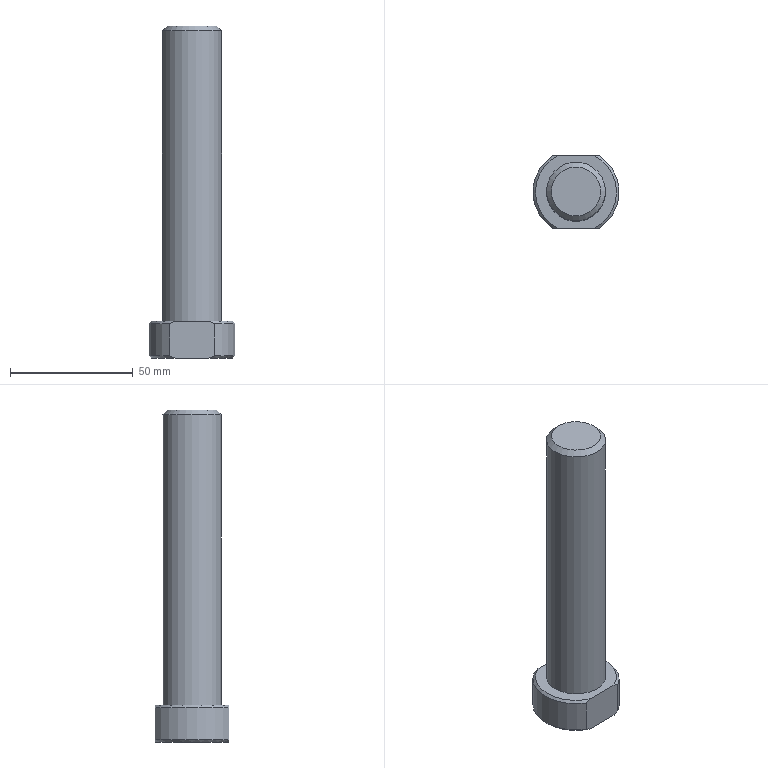Part | NX | features stopper pipe 2 | 1 solid | 13 faces | box 35 x 30 x 135 mm | volume 67591 mm3 | cone 5 | plane 5 | cylinder 3 | commonest cylinder face diameters 35 x2 24 x1
STEP:
#1=CARTESIAN_POINT('',(9.014,-15.,-1.));
#2=VERTEX_POINT('',#1);
#3=CARTESIAN_POINT('',(9.014,15.,-1.));
#4=VERTEX_POINT('',#3);
#5=CARTESIAN_POINT('',(0.,0.,-1.));
#6=DIRECTION('',(0.,0.,-1.));
#7=DIRECTION('',(-1.,0.,0.));
#8=AXIS2_PLACEMENT_3D('',#5,#6,#7);
#9=CIRCLE('',#8,17.5);
#10=EDGE_CURVE('',#2,#4,#9,.F.);
#11=ORIENTED_EDGE('',*,*,#10,.F.);
#12=CARTESIAN_POINT('',(9.014,-15.,-14.));
#13=VERTEX_POINT('',#12);
#14=CARTESIAN_POINT('',(9.014,-15.,120.));
#15=DIRECTION('',(0.,0.,-1.));
#16=VECTOR('',#15,1000.);
#17=LINE('',#14,#16);
#18=EDGE_CURVE('',#13,#2,#17,.F.);
#19=ORIENTED_EDGE('',*,*,#18,.F.);
#20=CARTESIAN_POINT('',(9.014,15.,-14.));
#21=VERTEX_POINT('',#20);
#22=CARTESIAN_POINT('',(0.,0.,-14.));
#23=DIRECTION('',(0.,0.,1.));
#24=DIRECTION('',(1.,0.,0.));
#25=AXIS2_PLACEMENT_3D('',#22,#23,#24);
#26=CIRCLE('',#25,17.5);
#27=EDGE_CURVE('',#21,#13,#26,.F.);
#28=ORIENTED_EDGE('',*,*,#27,.F.);
#29=CARTESIAN_POINT('',(9.014,15.,120.));
#30=DIRECTION('',(0.,0.,1.));
#31=VECTOR('',#30,1000.);
#32=LINE('',#29,#31);
#33=EDGE_CURVE('',#4,#21,#32,.F.);
#34=ORIENTED_EDGE('',*,*,#33,.F.);
#35=EDGE_LOOP('',(#11,#19,#28,#34));
#36=FACE_BOUND('',#35,.T.);
#37=CARTESIAN_POINT('',(0.,0.,-15.));
#38=DIRECTION('',(0.,0.,1.));
#39=DIRECTION('',(1.,0.,0.));
#40=AXIS2_PLACEMENT_3D('',#37,#38,#39);
#41=CYLINDRICAL_SURFACE('',#40,17.5);
#42=ADVANCED_FACE('',(#36),#41,.T.);
#43=CARTESIAN_POINT('',(-9.014,-15.,-1.));
#44=VERTEX_POINT('',#43);
#45=CARTESIAN_POINT('',(-9.014,-15.,-14.));
#46=VERTEX_POINT('',#45);
#47=CARTESIAN_POINT('',(-9.014,-15.,120.));
#48=DIRECTION('',(0.,0.,-1.));
#49=VECTOR('',#48,1000.);
#50=LINE('',#47,#49);
#51=EDGE_CURVE('',#44,#46,#50,.T.);
#52=ORIENTED_EDGE('',*,*,#51,.F.);
#53=CARTESIAN_POINT('',(-9.014,15.,-1.));
#54=VERTEX_POINT('',#53);
#55=CARTESIAN_POINT('',(0.,0.,-1.));
#56=DIRECTION('',(0.,0.,-1.));
#57=DIRECTION('',(-1.,0.,0.));
#58=AXIS2_PLACEMENT_3D('',#55,#56,#57);
#59=CIRCLE('',#58,17.5);
#60=EDGE_CURVE('',#54,#44,#59,.F.);
#61=ORIENTED_EDGE('',*,*,#60,.F.);
#62=CARTESIAN_POINT('',(-9.014,15.,-14.));
#63=VERTEX_POINT('',#62);
#64=CARTESIAN_POINT('',(-9.014,15.,120.));
#65=DIRECTION('',(0.,0.,1.));
#66=VECTOR('',#65,1000.);
#67=LINE('',#64,#66);
#68=EDGE_CURVE('',#63,#54,#67,.T.);
#69=ORIENTED_EDGE('',*,*,#68,.F.);
#70=CARTESIAN_POINT('',(0.,0.,-14.));
#71=DIRECTION('',(0.,0.,1.));
#72=DIRECTION('',(1.,0.,0.));
#73=AXIS2_PLACEMENT_3D('',#70,#71,#72);
#74=CIRCLE('',#73,17.5);
#75=EDGE_CURVE('',#46,#63,#74,.F.);
#76=ORIENTED_EDGE('',*,*,#75,.F.);
#77=EDGE_LOOP('',(#52,#61,#69,#76));
#78=FACE_BOUND('',#77,.T.);
#79=CARTESIAN_POINT('',(0.,0.,-15.));
#80=DIRECTION('',(0.,0.,1.));
#81=DIRECTION('',(1.,0.,0.));
#82=AXIS2_PLACEMENT_3D('',#79,#80,#81);
#83=CYLINDRICAL_SURFACE('',#82,17.5);
#84=ADVANCED_FACE('',(#78),#83,.T.);
#85=ORIENTED_EDGE('',*,*,#75,.T.);
#86=CARTESIAN_POINT('',(-6.874,15.,-15.));
#87=VERTEX_POINT('',#86);
#88=CARTESIAN_POINT('',(-6.874,15.,-15.));
#89=CARTESIAN_POINT('',(-7.601,15.,-14.697));
#90=CARTESIAN_POINT('',(-8.313,15.,-14.361));
#91=CARTESIAN_POINT('',(-9.014,15.,-14.));
#92=B_SPLINE_CURVE_WITH_KNOTS('',3,(#88,#89,#90,#91),.UNSPECIFIED.,.F.,.F.,(4,4),(0.,0.002362),.UNSPECIFIED.);
#93=EDGE_CURVE('',#87,#63,#92,.T.);
#94=ORIENTED_EDGE('',*,*,#93,.F.);
#95=CARTESIAN_POINT('',(-6.874,-15.,-15.));
#96=VERTEX_POINT('',#95);
#97=CARTESIAN_POINT('',(0.,0.,-15.));
#98=DIRECTION('',(0.,0.,1.));
#99=DIRECTION('',(0.,-1.,0.));
#100=AXIS2_PLACEMENT_3D('',#97,#98,#99);
#101=CIRCLE('',#100,16.5);
#102=EDGE_CURVE('',#96,#87,#101,.F.);
#103=ORIENTED_EDGE('',*,*,#102,.F.);
#104=CARTESIAN_POINT('',(-9.014,-15.,-14.));
#105=CARTESIAN_POINT('',(-8.313,-15.,-14.361));
#106=CARTESIAN_POINT('',(-7.601,-15.,-14.697));
#107=CARTESIAN_POINT('',(-6.874,-15.,-15.));
#108=B_SPLINE_CURVE_WITH_KNOTS('',3,(#104,#105,#106,#107),.UNSPECIFIED.,.F.,.F.,(4,4),(0.,0.002362),.UNSPECIFIED.);
#109=EDGE_CURVE('',#46,#96,#108,.T.);
#110=ORIENTED_EDGE('',*,*,#109,.F.);
#111=EDGE_LOOP('',(#85,#94,#103,#110));
#112=FACE_BOUND('',#111,.T.);
#113=CARTESIAN_POINT('',(0.,0.,-14.));
#114=DIRECTION('',(0.,0.,1.));
#115=DIRECTION('',(0.,-1.,0.));
#116=AXIS2_PLACEMENT_3D('',#113,#114,#115);
#117=CONICAL_SURFACE('',#116,17.5,0.7854);
#118=ADVANCED_FACE('',(#112),#117,.T.);
#119=ORIENTED_EDGE('',*,*,#102,.T.);
#120=CARTESIAN_POINT('',(6.874,15.,-15.));
#121=VERTEX_POINT('',#120);
#122=CARTESIAN_POINT('',(17.5,15.,-15.));
#123=DIRECTION('',(1.,0.,0.));
#124=VECTOR('',#123,1000.);
#125=LINE('',#122,#124);
#126=EDGE_CURVE('',#121,#87,#125,.F.);
#127=ORIENTED_EDGE('',*,*,#126,.F.);
#128=CARTESIAN_POINT('',(6.874,-15.,-15.));
#129=VERTEX_POINT('',#128);
#130=CARTESIAN_POINT('',(0.,0.,-15.));
#131=DIRECTION('',(0.,0.,1.));
#132=DIRECTION('',(0.,-1.,0.));
#133=AXIS2_PLACEMENT_3D('',#130,#131,#132);
#134=CIRCLE('',#133,16.5);
#135=EDGE_CURVE('',#129,#121,#134,.T.);
#136=ORIENTED_EDGE('',*,*,#135,.F.);
#137=CARTESIAN_POINT('',(17.5,-15.,-15.));
#138=DIRECTION('',(1.,0.,0.));
#139=VECTOR('',#138,1000.);
#140=LINE('',#137,#139);
#141=EDGE_CURVE('',#96,#129,#140,.T.);
#142=ORIENTED_EDGE('',*,*,#141,.F.);
#143=EDGE_LOOP('',(#119,#127,#136,#142));
#144=FACE_BOUND('',#143,.T.);
#145=CARTESIAN_POINT('',(0.,0.,-15.));
#146=DIRECTION('',(0.,0.,-1.));
#147=DIRECTION('',(-1.,0.,0.));
#148=AXIS2_PLACEMENT_3D('',#145,#146,#147);
#149=PLANE('',#148);
#150=ADVANCED_FACE('',(#144),#149,.T.);
#151=ORIENTED_EDGE('',*,*,#27,.T.);
#152=CARTESIAN_POINT('',(6.874,-15.,-15.));
#153=CARTESIAN_POINT('',(7.601,-15.,-14.697));
#154=CARTESIAN_POINT('',(8.313,-15.,-14.361));
#155=CARTESIAN_POINT('',(9.014,-15.,-14.));
#156=B_SPLINE_CURVE_WITH_KNOTS('',3,(#152,#153,#154,#155),.UNSPECIFIED.,.F.,.F.,(4,4),(0.,0.002362),.UNSPECIFIED.);
#157=EDGE_CURVE('',#129,#13,#156,.T.);
#158=ORIENTED_EDGE('',*,*,#157,.F.);
#159=ORIENTED_EDGE('',*,*,#135,.T.);
#160=CARTESIAN_POINT('',(9.014,15.,-14.));
#161=CARTESIAN_POINT('',(8.313,15.,-14.361));
#162=CARTESIAN_POINT('',(7.601,15.,-14.697));
#163=CARTESIAN_POINT('',(6.874,15.,-15.));
#164=B_SPLINE_CURVE_WITH_KNOTS('',3,(#160,#161,#162,#163),.UNSPECIFIED.,.F.,.F.,(4,4),(0.,0.002362),.UNSPECIFIED.);
#165=EDGE_CURVE('',#21,#121,#164,.T.);
#166=ORIENTED_EDGE('',*,*,#165,.F.);
#167=EDGE_LOOP('',(#151,#158,#159,#166));
#168=FACE_BOUND('',#167,.T.);
#169=CARTESIAN_POINT('',(0.,0.,-14.));
#170=DIRECTION('',(0.,0.,1.));
#171=DIRECTION('',(0.,-1.,0.));
#172=AXIS2_PLACEMENT_3D('',#169,#170,#171);
#173=CONICAL_SURFACE('',#172,17.5,0.7854);
#174=ADVANCED_FACE('',(#168),#173,.T.);
#175=CARTESIAN_POINT('',(-10.,0.,120.));
#176=VERTEX_POINT('',#175);
#177=CARTESIAN_POINT('',(0.,0.,120.));
#178=DIRECTION('',(0.,0.,-1.));
#179=DIRECTION('',(-1.,0.,0.));
#180=AXIS2_PLACEMENT_3D('',#177,#178,#179);
#181=CIRCLE('',#180,10.);
#182=EDGE_CURVE('',#176,#176,#181,.T.);
#183=ORIENTED_EDGE('',*,*,#182,.F.);
#184=EDGE_LOOP('',(#183));
#185=FACE_BOUND('',#184,.T.);
#186=CARTESIAN_POINT('',(0.,0.,120.));
#187=DIRECTION('',(0.,0.,1.));
#188=DIRECTION('',(1.,0.,0.));
#189=AXIS2_PLACEMENT_3D('',#186,#187,#188);
#190=PLANE('',#189);
#191=ADVANCED_FACE('',(#185),#190,.T.);
#192=CARTESIAN_POINT('',(-6.874,15.,0.));
#193=VERTEX_POINT('',#192);
#194=CARTESIAN_POINT('',(-9.014,15.,-1.));
#195=CARTESIAN_POINT('',(-8.313,15.,-0.6392));
#196=CARTESIAN_POINT('',(-7.601,15.,-0.3031));
#197=CARTESIAN_POINT('',(-6.874,15.,0.));
#198=B_SPLINE_CURVE_WITH_KNOTS('',3,(#194,#195,#196,#197),.UNSPECIFIED.,.F.,.F.,(4,4),(0.,0.002362),.UNSPECIFIED.);
#199=EDGE_CURVE('',#54,#193,#198,.T.);
#200=ORIENTED_EDGE('',*,*,#199,.F.);
#201=ORIENTED_EDGE('',*,*,#60,.T.);
#202=CARTESIAN_POINT('',(-6.874,-15.,0.));
#203=VERTEX_POINT('',#202);
#204=CARTESIAN_POINT('',(-6.874,-15.,0.));
#205=CARTESIAN_POINT('',(-7.601,-15.,-0.3031));
#206=CARTESIAN_POINT('',(-8.313,-15.,-0.6392));
#207=CARTESIAN_POINT('',(-9.014,-15.,-1.));
#208=B_SPLINE_CURVE_WITH_KNOTS('',3,(#204,#205,#206,#207),.UNSPECIFIED.,.F.,.F.,(4,4),(0.,0.002362),.UNSPECIFIED.);
#209=EDGE_CURVE('',#203,#44,#208,.T.);
#210=ORIENTED_EDGE('',*,*,#209,.F.);
#211=CARTESIAN_POINT('',(0.,0.,0.));
#212=DIRECTION('',(0.,0.,-1.));
#213=DIRECTION('',(-1.,0.,0.));
#214=AXIS2_PLACEMENT_3D('',#211,#212,#213);
#215=CIRCLE('',#214,16.5);
#216=EDGE_CURVE('',#203,#193,#215,.T.);
#217=ORIENTED_EDGE('',*,*,#216,.T.);
#218=EDGE_LOOP('',(#200,#201,#210,#217));
#219=FACE_BOUND('',#218,.T.);
#220=CARTESIAN_POINT('',(0.,0.,-1.));
#221=DIRECTION('',(0.,0.,-1.));
#222=DIRECTION('',(-1.,0.,0.));
#223=AXIS2_PLACEMENT_3D('',#220,#221,#222);
#224=CONICAL_SURFACE('',#223,17.5,0.7854);
#225=ADVANCED_FACE('',(#219),#224,.T.);
#226=ORIENTED_EDGE('',*,*,#126,.T.);
#227=ORIENTED_EDGE('',*,*,#93,.T.);
#228=ORIENTED_EDGE('',*,*,#68,.T.);
#229=ORIENTED_EDGE('',*,*,#199,.T.);
#230=CARTESIAN_POINT('',(6.874,15.,0.));
#231=VERTEX_POINT('',#230);
#232=CARTESIAN_POINT('',(0.,15.,0.));
#233=DIRECTION('',(-1.,0.,0.));
#234=VECTOR('',#233,1000.);
#235=LINE('',#232,#234);
#236=EDGE_CURVE('',#193,#231,#235,.F.);
#237=ORIENTED_EDGE('',*,*,#236,.T.);
#238=CARTESIAN_POINT('',(9.014,15.,-1.));
#239=CARTESIAN_POINT('',(8.313,15.,-0.6392));
#240=CARTESIAN_POINT('',(7.601,15.,-0.3031));
#241=CARTESIAN_POINT('',(6.874,15.,0.));
#242=B_SPLINE_CURVE_WITH_KNOTS('',3,(#238,#239,#240,#241),.UNSPECIFIED.,.F.,.F.,(4,4),(0.,0.002362),.UNSPECIFIED.);
#243=EDGE_CURVE('',#4,#231,#242,.T.);
#244=ORIENTED_EDGE('',*,*,#243,.F.);
#245=ORIENTED_EDGE('',*,*,#33,.T.);
#246=ORIENTED_EDGE('',*,*,#165,.T.);
#247=EDGE_LOOP('',(#226,#227,#228,#229,#237,#244,#245,#246));
#248=FACE_BOUND('',#247,.T.);
#249=CARTESIAN_POINT('',(17.5,15.,120.));
#250=DIRECTION('',(0.,1.,0.));
#251=DIRECTION('',(0.,0.,1.));
#252=AXIS2_PLACEMENT_3D('',#249,#250,#251);
#253=PLANE('',#252);
#254=ADVANCED_FACE('',(#248),#253,.T.);
#255=ORIENTED_EDGE('',*,*,#10,.T.);
#256=ORIENTED_EDGE('',*,*,#243,.T.);
#257=CARTESIAN_POINT('',(6.874,-15.,0.));
#258=VERTEX_POINT('',#257);
#259=CARTESIAN_POINT('',(0.,0.,0.));
#260=DIRECTION('',(0.,0.,-1.));
#261=DIRECTION('',(-1.,0.,0.));
#262=AXIS2_PLACEMENT_3D('',#259,#260,#261);
#263=CIRCLE('',#262,16.5);
#264=EDGE_CURVE('',#231,#258,#263,.T.);
#265=ORIENTED_EDGE('',*,*,#264,.T.);
#266=CARTESIAN_POINT('',(9.014,-15.,-1.));
#267=CARTESIAN_POINT('',(8.313,-15.,-0.6392));
#268=CARTESIAN_POINT('',(7.601,-15.,-0.3031));
#269=CARTESIAN_POINT('',(6.874,-15.,0.));
#270=B_SPLINE_CURVE_WITH_KNOTS('',3,(#266,#267,#268,#269),.UNSPECIFIED.,.F.,.F.,(4,4),(0.,0.002362),.UNSPECIFIED.);
#271=EDGE_CURVE('',#2,#258,#270,.T.);
#272=ORIENTED_EDGE('',*,*,#271,.F.);
#273=EDGE_LOOP('',(#255,#256,#265,#272));
#274=FACE_BOUND('',#273,.T.);
#275=CARTESIAN_POINT('',(0.,0.,-1.));
#276=DIRECTION('',(0.,0.,-1.));
#277=DIRECTION('',(-1.,0.,0.));
#278=AXIS2_PLACEMENT_3D('',#275,#276,#277);
#279=CONICAL_SURFACE('',#278,17.5,0.7854);
#280=ADVANCED_FACE('',(#274),#279,.T.);
#281=ORIENTED_EDGE('',*,*,#141,.T.);
#282=ORIENTED_EDGE('',*,*,#157,.T.);
#283=ORIENTED_EDGE('',*,*,#18,.T.);
#284=ORIENTED_EDGE('',*,*,#271,.T.);
#285=CARTESIAN_POINT('',(0.,-15.,0.));
#286=DIRECTION('',(-1.,0.,0.));
#287=VECTOR('',#286,1000.);
#288=LINE('',#285,#287);
#289=EDGE_CURVE('',#258,#203,#288,.T.);
#290=ORIENTED_EDGE('',*,*,#289,.T.);
#291=ORIENTED_EDGE('',*,*,#209,.T.);
#292=ORIENTED_EDGE('',*,*,#51,.T.);
#293=ORIENTED_EDGE('',*,*,#109,.T.);
#294=EDGE_LOOP('',(#281,#282,#283,#284,#290,#291,#292,#293));
#295=FACE_BOUND('',#294,.T.);
#296=CARTESIAN_POINT('',(17.5,-15.,120.));
#297=DIRECTION('',(0.,-1.,0.));
#298=DIRECTION('',(0.,0.,-1.));
#299=AXIS2_PLACEMENT_3D('',#296,#297,#298);
#300=PLANE('',#299);
#301=ADVANCED_FACE('',(#295),#300,.T.);
#302=CARTESIAN_POINT('',(-12.,0.,118.));
#303=VERTEX_POINT('',#302);
#304=CARTESIAN_POINT('',(0.,0.,118.));
#305=DIRECTION('',(0.,0.,-1.));
#306=DIRECTION('',(-1.,0.,0.));
#307=AXIS2_PLACEMENT_3D('',#304,#305,#306);
#308=CIRCLE('',#307,12.);
#309=EDGE_CURVE('',#303,#303,#308,.T.);
#310=ORIENTED_EDGE('',*,*,#309,.F.);
#311=EDGE_LOOP('',(#310));
#312=FACE_BOUND('',#311,.T.);
#313=ORIENTED_EDGE('',*,*,#182,.T.);
#314=EDGE_LOOP('',(#313));
#315=FACE_BOUND('',#314,.T.);
#316=CARTESIAN_POINT('',(0.,0.,118.));
#317=DIRECTION('',(0.,0.,-1.));
#318=DIRECTION('',(-1.,0.,0.));
#319=AXIS2_PLACEMENT_3D('',#316,#317,#318);
#320=CONICAL_SURFACE('',#319,12.,0.7854);
#321=ADVANCED_FACE('',(#312,#315),#320,.T.);
#322=ORIENTED_EDGE('',*,*,#264,.F.);
#323=ORIENTED_EDGE('',*,*,#236,.F.);
#324=ORIENTED_EDGE('',*,*,#216,.F.);
#325=ORIENTED_EDGE('',*,*,#289,.F.);
#326=EDGE_LOOP('',(#322,#323,#324,#325));
#327=FACE_BOUND('',#326,.T.);
#328=CARTESIAN_POINT('',(-12.,0.,0.));
#329=VERTEX_POINT('',#328);
#330=CARTESIAN_POINT('',(0.,0.,0.));
#331=DIRECTION('',(0.,0.,-1.));
#332=DIRECTION('',(-1.,0.,0.));
#333=AXIS2_PLACEMENT_3D('',#330,#331,#332);
#334=CIRCLE('',#333,12.);
#335=EDGE_CURVE('',#329,#329,#334,.F.);
#336=ORIENTED_EDGE('',*,*,#335,.F.);
#337=EDGE_LOOP('',(#336));
#338=FACE_BOUND('',#337,.T.);
#339=CARTESIAN_POINT('',(0.,0.,0.));
#340=DIRECTION('',(0.,0.,-1.));
#341=DIRECTION('',(-1.,0.,0.));
#342=AXIS2_PLACEMENT_3D('',#339,#340,#341);
#343=PLANE('',#342);
#344=ADVANCED_FACE('',(#327,#338),#343,.F.);
#345=ORIENTED_EDGE('',*,*,#335,.T.);
#346=EDGE_LOOP('',(#345));
#347=FACE_BOUND('',#346,.T.);
#348=ORIENTED_EDGE('',*,*,#309,.T.);
#349=EDGE_LOOP('',(#348));
#350=FACE_BOUND('',#349,.T.);
#351=CARTESIAN_POINT('',(0.,0.,120.));
#352=DIRECTION('',(0.,0.,-1.));
#353=DIRECTION('',(-1.,0.,0.));
#354=AXIS2_PLACEMENT_3D('',#351,#352,#353);
#355=CYLINDRICAL_SURFACE('',#354,12.);
#356=ADVANCED_FACE('',(#347,#350),#355,.T.);
#357=CLOSED_SHELL('',(#42,#84,#118,#150,#174,#191,#225,#254,#280,#301,#321,#344,#356));
#358=MANIFOLD_SOLID_BREP('',#357);
#359=(LENGTH_UNIT()NAMED_UNIT(*)SI_UNIT(.MILLI.,.METRE.));
#360=UNCERTAINTY_MEASURE_WITH_UNIT(LENGTH_MEASURE(0.0508),#359,'','');
#361=(NAMED_UNIT(*)PLANE_ANGLE_UNIT()SI_UNIT($,.RADIAN.));
#362=(NAMED_UNIT(*)SI_UNIT($,.STERADIAN.)SOLID_ANGLE_UNIT());
#363=(GEOMETRIC_REPRESENTATION_CONTEXT(3)GLOBAL_UNCERTAINTY_ASSIGNED_CONTEXT((#360))GLOBAL_UNIT_ASSIGNED_CONTEXT((#359,#361,#362))REPRESENTATION_CONTEXT('',''));
#364=ADVANCED_BREP_SHAPE_REPRESENTATION('',(#358),#363);